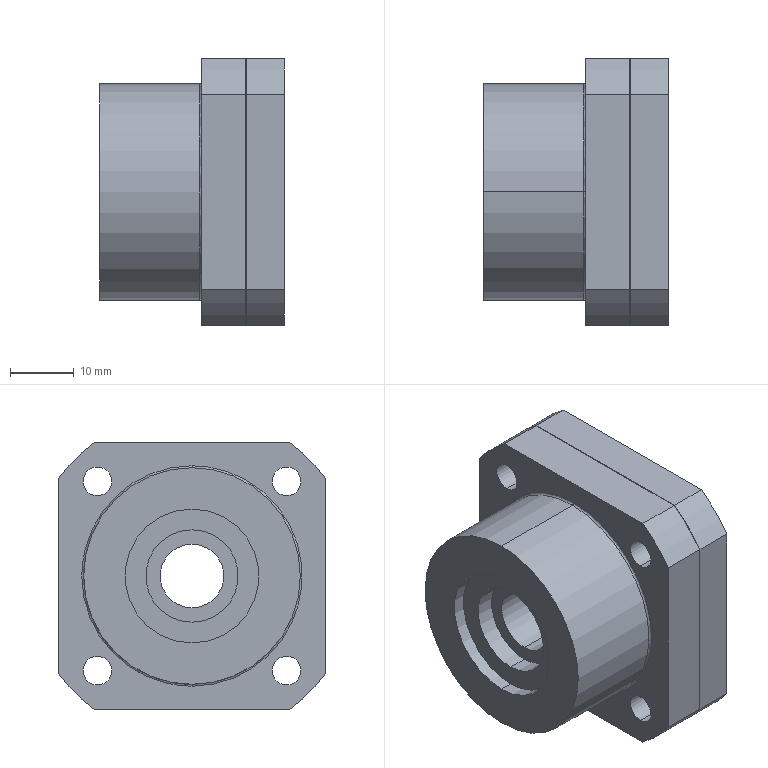Part | SolidWorks | features BaseBody 1 | 1 solid | 122 faces | box 29 x 42 x 42 mm | volume 30074 mm3 | plane 62 | cylinder 58 | spline 2 | commonest cylinder face diameters 4.5 x8 6.2 x8 7 x8 8 x8 52 x8 14.5 x4